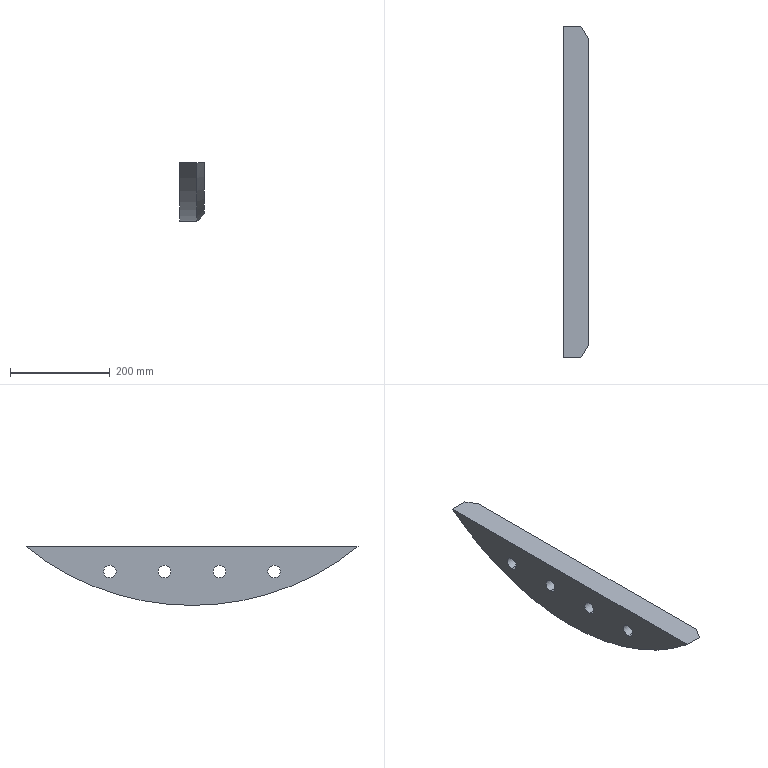Part | SolidWorks | features Chamfer 1, Extrusion 1, ICE 1 | 1 solid | 13 faces | box 50 x 666.801 x 118 mm | volume 2510197 mm3 | cylinder 9 | plane 3 | cone 1 | commonest cylinder face diameters 25 x8 1060 x1
STEP:
#1=CARTESIAN_POINT('',(-25.,-165.,-449.5));
#2=VERTEX_POINT('',#1);
#3=CARTESIAN_POINT('',(-25.,-165.,-474.5));
#4=VERTEX_POINT('',#3);
#5=CARTESIAN_POINT('',(-25.,-165.,-462.));
#6=DIRECTION('',(1.,0.,0.));
#7=DIRECTION('',(0.,0.,-1.));
#8=AXIS2_PLACEMENT_3D('',#5,#6,#7);
#9=CIRCLE('',#8,12.5);
#10=EDGE_CURVE('',#2,#4,#9,.T.);
#11=ORIENTED_EDGE('',*,*,#10,.F.);
#12=CARTESIAN_POINT('',(25.,-165.,-449.5));
#13=VERTEX_POINT('',#12);
#14=CARTESIAN_POINT('',(-56.,-165.,-449.5));
#15=DIRECTION('',(1.,0.,0.));
#16=VECTOR('',#15,1000.);
#17=LINE('',#14,#16);
#18=EDGE_CURVE('',#2,#13,#17,.T.);
#19=ORIENTED_EDGE('',*,*,#18,.T.);
#20=CARTESIAN_POINT('',(25.,-165.,-474.5));
#21=VERTEX_POINT('',#20);
#22=CARTESIAN_POINT('',(25.,-165.,-462.));
#23=DIRECTION('',(1.,0.,0.));
#24=DIRECTION('',(0.,0.,-1.));
#25=AXIS2_PLACEMENT_3D('',#22,#23,#24);
#26=CIRCLE('',#25,12.5);
#27=EDGE_CURVE('',#13,#21,#26,.T.);
#28=ORIENTED_EDGE('',*,*,#27,.T.);
#29=CARTESIAN_POINT('',(-56.,-165.,-474.5));
#30=DIRECTION('',(1.,0.,0.));
#31=VECTOR('',#30,1000.);
#32=LINE('',#29,#31);
#33=EDGE_CURVE('',#4,#21,#32,.T.);
#34=ORIENTED_EDGE('',*,*,#33,.F.);
#35=EDGE_LOOP('',(#11,#19,#28,#34));
#36=FACE_OUTER_BOUND('',#35,.T.);
#37=CARTESIAN_POINT('',(-56.,-165.,-462.));
#38=DIRECTION('',(1.,0.,0.));
#39=DIRECTION('',(0.,0.,-1.));
#40=AXIS2_PLACEMENT_3D('',#37,#38,#39);
#41=CYLINDRICAL_SURFACE('',#40,12.5);
#42=ADVANCED_FACE('',(#36),#41,.F.);
#43=CARTESIAN_POINT('',(-25.,165.,-449.5));
#44=VERTEX_POINT('',#43);
#45=CARTESIAN_POINT('',(-25.,165.,-474.5));
#46=VERTEX_POINT('',#45);
#47=CARTESIAN_POINT('',(-25.,165.,-462.));
#48=DIRECTION('',(1.,0.,0.));
#49=DIRECTION('',(0.,0.,-1.));
#50=AXIS2_PLACEMENT_3D('',#47,#48,#49);
#51=CIRCLE('',#50,12.5);
#52=EDGE_CURVE('',#44,#46,#51,.T.);
#53=ORIENTED_EDGE('',*,*,#52,.F.);
#54=CARTESIAN_POINT('',(25.,165.,-449.5));
#55=VERTEX_POINT('',#54);
#56=CARTESIAN_POINT('',(-56.,165.,-449.5));
#57=DIRECTION('',(1.,0.,0.));
#58=VECTOR('',#57,1000.);
#59=LINE('',#56,#58);
#60=EDGE_CURVE('',#44,#55,#59,.T.);
#61=ORIENTED_EDGE('',*,*,#60,.T.);
#62=CARTESIAN_POINT('',(25.,165.,-474.5));
#63=VERTEX_POINT('',#62);
#64=CARTESIAN_POINT('',(25.,165.,-462.));
#65=DIRECTION('',(1.,0.,0.));
#66=DIRECTION('',(0.,0.,-1.));
#67=AXIS2_PLACEMENT_3D('',#64,#65,#66);
#68=CIRCLE('',#67,12.5);
#69=EDGE_CURVE('',#55,#63,#68,.T.);
#70=ORIENTED_EDGE('',*,*,#69,.T.);
#71=CARTESIAN_POINT('',(-56.,165.,-474.5));
#72=DIRECTION('',(1.,0.,0.));
#73=VECTOR('',#72,1000.);
#74=LINE('',#71,#73);
#75=EDGE_CURVE('',#46,#63,#74,.T.);
#76=ORIENTED_EDGE('',*,*,#75,.F.);
#77=EDGE_LOOP('',(#53,#61,#70,#76));
#78=FACE_OUTER_BOUND('',#77,.T.);
#79=CARTESIAN_POINT('',(-56.,165.,-462.));
#80=DIRECTION('',(1.,0.,0.));
#81=DIRECTION('',(0.,0.,-1.));
#82=AXIS2_PLACEMENT_3D('',#79,#80,#81);
#83=CYLINDRICAL_SURFACE('',#82,12.5);
#84=ADVANCED_FACE('',(#78),#83,.F.);
#85=CARTESIAN_POINT('',(-25.,-55.,-449.5));
#86=VERTEX_POINT('',#85);
#87=CARTESIAN_POINT('',(-25.,-55.,-474.5));
#88=VERTEX_POINT('',#87);
#89=CARTESIAN_POINT('',(-25.,-55.,-462.));
#90=DIRECTION('',(1.,0.,0.));
#91=DIRECTION('',(0.,0.,-1.));
#92=AXIS2_PLACEMENT_3D('',#89,#90,#91);
#93=CIRCLE('',#92,12.5);
#94=EDGE_CURVE('',#86,#88,#93,.T.);
#95=ORIENTED_EDGE('',*,*,#94,.F.);
#96=CARTESIAN_POINT('',(25.,-55.,-449.5));
#97=VERTEX_POINT('',#96);
#98=CARTESIAN_POINT('',(-56.,-55.,-449.5));
#99=DIRECTION('',(1.,0.,0.));
#100=VECTOR('',#99,1000.);
#101=LINE('',#98,#100);
#102=EDGE_CURVE('',#86,#97,#101,.T.);
#103=ORIENTED_EDGE('',*,*,#102,.T.);
#104=CARTESIAN_POINT('',(25.,-55.,-474.5));
#105=VERTEX_POINT('',#104);
#106=CARTESIAN_POINT('',(25.,-55.,-462.));
#107=DIRECTION('',(1.,0.,0.));
#108=DIRECTION('',(0.,0.,-1.));
#109=AXIS2_PLACEMENT_3D('',#106,#107,#108);
#110=CIRCLE('',#109,12.5);
#111=EDGE_CURVE('',#97,#105,#110,.T.);
#112=ORIENTED_EDGE('',*,*,#111,.T.);
#113=CARTESIAN_POINT('',(-56.,-55.,-474.5));
#114=DIRECTION('',(1.,0.,0.));
#115=VECTOR('',#114,1000.);
#116=LINE('',#113,#115);
#117=EDGE_CURVE('',#88,#105,#116,.T.);
#118=ORIENTED_EDGE('',*,*,#117,.F.);
#119=EDGE_LOOP('',(#95,#103,#112,#118));
#120=FACE_OUTER_BOUND('',#119,.T.);
#121=CARTESIAN_POINT('',(-56.,-55.,-462.));
#122=DIRECTION('',(1.,0.,0.));
#123=DIRECTION('',(0.,0.,-1.));
#124=AXIS2_PLACEMENT_3D('',#121,#122,#123);
#125=CYLINDRICAL_SURFACE('',#124,12.5);
#126=ADVANCED_FACE('',(#120),#125,.F.);
#127=CARTESIAN_POINT('',(-25.,55.,-449.5));
#128=VERTEX_POINT('',#127);
#129=CARTESIAN_POINT('',(-25.,55.,-474.5));
#130=VERTEX_POINT('',#129);
#131=CARTESIAN_POINT('',(-25.,55.,-462.));
#132=DIRECTION('',(1.,0.,0.));
#133=DIRECTION('',(0.,0.,-1.));
#134=AXIS2_PLACEMENT_3D('',#131,#132,#133);
#135=CIRCLE('',#134,12.5);
#136=EDGE_CURVE('',#128,#130,#135,.T.);
#137=ORIENTED_EDGE('',*,*,#136,.F.);
#138=CARTESIAN_POINT('',(25.,55.,-449.5));
#139=VERTEX_POINT('',#138);
#140=CARTESIAN_POINT('',(-56.,55.,-449.5));
#141=DIRECTION('',(1.,0.,0.));
#142=VECTOR('',#141,1000.);
#143=LINE('',#140,#142);
#144=EDGE_CURVE('',#128,#139,#143,.T.);
#145=ORIENTED_EDGE('',*,*,#144,.T.);
#146=CARTESIAN_POINT('',(25.,55.,-474.5));
#147=VERTEX_POINT('',#146);
#148=CARTESIAN_POINT('',(25.,55.,-462.));
#149=DIRECTION('',(1.,0.,0.));
#150=DIRECTION('',(0.,0.,-1.));
#151=AXIS2_PLACEMENT_3D('',#148,#149,#150);
#152=CIRCLE('',#151,12.5);
#153=EDGE_CURVE('',#139,#147,#152,.T.);
#154=ORIENTED_EDGE('',*,*,#153,.T.);
#155=CARTESIAN_POINT('',(-56.,55.,-474.5));
#156=DIRECTION('',(1.,0.,0.));
#157=VECTOR('',#156,1000.);
#158=LINE('',#155,#157);
#159=EDGE_CURVE('',#130,#147,#158,.T.);
#160=ORIENTED_EDGE('',*,*,#159,.F.);
#161=EDGE_LOOP('',(#137,#145,#154,#160));
#162=FACE_OUTER_BOUND('',#161,.T.);
#163=CARTESIAN_POINT('',(-56.,55.,-462.));
#164=DIRECTION('',(1.,0.,0.));
#165=DIRECTION('',(0.,0.,-1.));
#166=AXIS2_PLACEMENT_3D('',#163,#164,#165);
#167=CYLINDRICAL_SURFACE('',#166,12.5);
#168=ADVANCED_FACE('',(#162),#167,.F.);
#169=CARTESIAN_POINT('',(10.,333.401,-412.));
#170=VERTEX_POINT('',#169);
#171=CARTESIAN_POINT('',(-25.,333.401,-412.));
#172=VERTEX_POINT('',#171);
#173=CARTESIAN_POINT('',(25.,333.401,-412.));
#174=DIRECTION('',(-1.,0.,0.));
#175=VECTOR('',#174,1000.);
#176=LINE('',#173,#175);
#177=EDGE_CURVE('',#170,#172,#176,.T.);
#178=ORIENTED_EDGE('',*,*,#177,.F.);
#179=CARTESIAN_POINT('',(10.,-333.401,-412.));
#180=VERTEX_POINT('',#179);
#181=CARTESIAN_POINT('',(10.,0.,0.));
#182=DIRECTION('',(-1.,0.,0.));
#183=DIRECTION('',(0.,0.,-1.));
#184=AXIS2_PLACEMENT_3D('',#181,#182,#183);
#185=CIRCLE('',#184,530.);
#186=EDGE_CURVE('',#170,#180,#185,.T.);
#187=ORIENTED_EDGE('',*,*,#186,.T.);
#188=CARTESIAN_POINT('',(-25.,-333.401,-412.));
#189=VERTEX_POINT('',#188);
#190=CARTESIAN_POINT('',(25.,-333.401,-412.));
#191=DIRECTION('',(-1.,0.,0.));
#192=VECTOR('',#191,1000.);
#193=LINE('',#190,#192);
#194=EDGE_CURVE('',#180,#189,#193,.T.);
#195=ORIENTED_EDGE('',*,*,#194,.T.);
#196=CARTESIAN_POINT('',(-25.,0.,0.));
#197=DIRECTION('',(1.,0.,0.));
#198=DIRECTION('',(0.,0.,-1.));
#199=AXIS2_PLACEMENT_3D('',#196,#197,#198);
#200=CIRCLE('',#199,530.);
#201=EDGE_CURVE('',#189,#172,#200,.T.);
#202=ORIENTED_EDGE('',*,*,#201,.T.);
#203=EDGE_LOOP('',(#178,#187,#195,#202));
#204=FACE_OUTER_BOUND('',#203,.T.);
#205=CARTESIAN_POINT('',(25.,0.,0.));
#206=DIRECTION('',(-1.,0.,0.));
#207=DIRECTION('',(0.,0.,1.));
#208=AXIS2_PLACEMENT_3D('',#205,#206,#207);
#209=CYLINDRICAL_SURFACE('',#208,530.);
#210=ADVANCED_FACE('',(#204),#209,.T.);
#211=CARTESIAN_POINT('',(25.,309.,-412.));
#212=VERTEX_POINT('',#211);
#213=CARTESIAN_POINT('',(25.,-309.,-412.));
#214=VERTEX_POINT('',#213);
#215=CARTESIAN_POINT('',(25.,333.401,-412.));
#216=DIRECTION('',(0.,-1.,0.));
#217=VECTOR('',#216,1000.);
#218=LINE('',#215,#217);
#219=EDGE_CURVE('',#212,#214,#218,.T.);
#220=ORIENTED_EDGE('',*,*,#219,.F.);
#221=CARTESIAN_POINT('',(25.,309.,-412.));
#222=CARTESIAN_POINT('',(20.088,317.187,-412.));
#223=CARTESIAN_POINT('',(15.084,325.319,-412.));
#224=CARTESIAN_POINT('',(10.,333.401,-412.));
#225=B_SPLINE_CURVE_WITH_KNOTS('',3,(#221,#222,#223,#224),.UNSPECIFIED.,.F.,.F.,(4,4),(0.,0.02864),.UNSPECIFIED.);
#226=EDGE_CURVE('',#212,#170,#225,.T.);
#227=ORIENTED_EDGE('',*,*,#226,.T.);
#228=ORIENTED_EDGE('',*,*,#177,.T.);
#229=CARTESIAN_POINT('',(-25.,333.401,-412.));
#230=DIRECTION('',(0.,-1.,0.));
#231=VECTOR('',#230,1000.);
#232=LINE('',#229,#231);
#233=EDGE_CURVE('',#172,#189,#232,.T.);
#234=ORIENTED_EDGE('',*,*,#233,.T.);
#235=ORIENTED_EDGE('',*,*,#194,.F.);
#236=CARTESIAN_POINT('',(10.,-333.401,-412.));
#237=CARTESIAN_POINT('',(15.084,-325.319,-412.));
#238=CARTESIAN_POINT('',(20.088,-317.187,-412.));
#239=CARTESIAN_POINT('',(25.,-309.,-412.));
#240=B_SPLINE_CURVE_WITH_KNOTS('',3,(#236,#237,#238,#239),.UNSPECIFIED.,.F.,.F.,(4,4),(0.,0.02864),.UNSPECIFIED.);
#241=EDGE_CURVE('',#180,#214,#240,.T.);
#242=ORIENTED_EDGE('',*,*,#241,.T.);
#243=EDGE_LOOP('',(#220,#227,#228,#234,#235,#242));
#244=FACE_OUTER_BOUND('',#243,.T.);
#245=CARTESIAN_POINT('',(25.,333.401,-412.));
#246=DIRECTION('',(0.,0.,-1.));
#247=DIRECTION('',(-1.,0.,0.));
#248=AXIS2_PLACEMENT_3D('',#245,#246,#247);
#249=PLANE('',#248);
#250=ADVANCED_FACE('',(#244),#249,.F.);
#251=CARTESIAN_POINT('',(25.,-165.,-462.));
#252=DIRECTION('',(1.,0.,0.));
#253=DIRECTION('',(0.,0.,-1.));
#254=AXIS2_PLACEMENT_3D('',#251,#252,#253);
#255=CIRCLE('',#254,12.5);
#256=EDGE_CURVE('',#21,#13,#255,.T.);
#257=ORIENTED_EDGE('',*,*,#256,.F.);
#258=ORIENTED_EDGE('',*,*,#27,.F.);
#259=EDGE_LOOP('',(#257,#258));
#260=FACE_BOUND('',#259,.T.);
#261=CARTESIAN_POINT('',(25.,165.,-462.));
#262=DIRECTION('',(1.,0.,0.));
#263=DIRECTION('',(0.,0.,-1.));
#264=AXIS2_PLACEMENT_3D('',#261,#262,#263);
#265=CIRCLE('',#264,12.5);
#266=EDGE_CURVE('',#63,#55,#265,.T.);
#267=ORIENTED_EDGE('',*,*,#266,.F.);
#268=ORIENTED_EDGE('',*,*,#69,.F.);
#269=EDGE_LOOP('',(#267,#268));
#270=FACE_BOUND('',#269,.T.);
#271=CARTESIAN_POINT('',(25.,-55.,-462.));
#272=DIRECTION('',(1.,0.,0.));
#273=DIRECTION('',(0.,0.,-1.));
#274=AXIS2_PLACEMENT_3D('',#271,#272,#273);
#275=CIRCLE('',#274,12.5);
#276=EDGE_CURVE('',#105,#97,#275,.T.);
#277=ORIENTED_EDGE('',*,*,#276,.F.);
#278=ORIENTED_EDGE('',*,*,#111,.F.);
#279=EDGE_LOOP('',(#277,#278));
#280=FACE_BOUND('',#279,.T.);
#281=CARTESIAN_POINT('',(25.,55.,-462.));
#282=DIRECTION('',(1.,0.,0.));
#283=DIRECTION('',(0.,0.,-1.));
#284=AXIS2_PLACEMENT_3D('',#281,#282,#283);
#285=CIRCLE('',#284,12.5);
#286=EDGE_CURVE('',#147,#139,#285,.T.);
#287=ORIENTED_EDGE('',*,*,#286,.F.);
#288=ORIENTED_EDGE('',*,*,#153,.F.);
#289=EDGE_LOOP('',(#287,#288));
#290=FACE_BOUND('',#289,.T.);
#291=ORIENTED_EDGE('',*,*,#219,.T.);
#292=CARTESIAN_POINT('',(25.,0.,0.));
#293=DIRECTION('',(1.,0.,0.));
#294=DIRECTION('',(0.,0.,-1.));
#295=AXIS2_PLACEMENT_3D('',#292,#293,#294);
#296=CIRCLE('',#295,515.);
#297=EDGE_CURVE('',#214,#212,#296,.T.);
#298=ORIENTED_EDGE('',*,*,#297,.T.);
#299=EDGE_LOOP('',(#291,#298));
#300=FACE_OUTER_BOUND('',#299,.T.);
#301=CARTESIAN_POINT('',(25.,0.,0.));
#302=DIRECTION('',(1.,0.,0.));
#303=DIRECTION('',(0.,0.,-1.));
#304=AXIS2_PLACEMENT_3D('',#301,#302,#303);
#305=PLANE('',#304);
#306=ADVANCED_FACE('',(#260,#270,#280,#290,#300),#305,.T.);
#307=CARTESIAN_POINT('',(-25.,-165.,-462.));
#308=DIRECTION('',(1.,0.,0.));
#309=DIRECTION('',(0.,0.,-1.));
#310=AXIS2_PLACEMENT_3D('',#307,#308,#309);
#311=CIRCLE('',#310,12.5);
#312=EDGE_CURVE('',#4,#2,#311,.T.);
#313=ORIENTED_EDGE('',*,*,#312,.T.);
#314=ORIENTED_EDGE('',*,*,#10,.T.);
#315=EDGE_LOOP('',(#313,#314));
#316=FACE_BOUND('',#315,.T.);
#317=CARTESIAN_POINT('',(-25.,165.,-462.));
#318=DIRECTION('',(1.,0.,0.));
#319=DIRECTION('',(0.,0.,-1.));
#320=AXIS2_PLACEMENT_3D('',#317,#318,#319);
#321=CIRCLE('',#320,12.5);
#322=EDGE_CURVE('',#46,#44,#321,.T.);
#323=ORIENTED_EDGE('',*,*,#322,.T.);
#324=ORIENTED_EDGE('',*,*,#52,.T.);
#325=EDGE_LOOP('',(#323,#324));
#326=FACE_BOUND('',#325,.T.);
#327=CARTESIAN_POINT('',(-25.,-55.,-462.));
#328=DIRECTION('',(1.,0.,0.));
#329=DIRECTION('',(0.,0.,-1.));
#330=AXIS2_PLACEMENT_3D('',#327,#328,#329);
#331=CIRCLE('',#330,12.5);
#332=EDGE_CURVE('',#88,#86,#331,.T.);
#333=ORIENTED_EDGE('',*,*,#332,.T.);
#334=ORIENTED_EDGE('',*,*,#94,.T.);
#335=EDGE_LOOP('',(#333,#334));
#336=FACE_BOUND('',#335,.T.);
#337=CARTESIAN_POINT('',(-25.,55.,-462.));
#338=DIRECTION('',(1.,0.,0.));
#339=DIRECTION('',(0.,0.,-1.));
#340=AXIS2_PLACEMENT_3D('',#337,#338,#339);
#341=CIRCLE('',#340,12.5);
#342=EDGE_CURVE('',#130,#128,#341,.T.);
#343=ORIENTED_EDGE('',*,*,#342,.T.);
#344=ORIENTED_EDGE('',*,*,#136,.T.);
#345=EDGE_LOOP('',(#343,#344));
#346=FACE_BOUND('',#345,.T.);
#347=ORIENTED_EDGE('',*,*,#201,.F.);
#348=ORIENTED_EDGE('',*,*,#233,.F.);
#349=EDGE_LOOP('',(#347,#348));
#350=FACE_OUTER_BOUND('',#349,.T.);
#351=CARTESIAN_POINT('',(-25.,0.,0.));
#352=DIRECTION('',(1.,0.,0.));
#353=DIRECTION('',(0.,0.,-1.));
#354=AXIS2_PLACEMENT_3D('',#351,#352,#353);
#355=PLANE('',#354);
#356=ADVANCED_FACE('',(#316,#326,#336,#346,#350),#355,.F.);
#357=ORIENTED_EDGE('',*,*,#144,.F.);
#358=ORIENTED_EDGE('',*,*,#342,.F.);
#359=ORIENTED_EDGE('',*,*,#159,.T.);
#360=ORIENTED_EDGE('',*,*,#286,.T.);
#361=EDGE_LOOP('',(#357,#358,#359,#360));
#362=FACE_OUTER_BOUND('',#361,.T.);
#363=CARTESIAN_POINT('',(-56.,55.,-462.));
#364=DIRECTION('',(1.,0.,0.));
#365=DIRECTION('',(0.,0.,-1.));
#366=AXIS2_PLACEMENT_3D('',#363,#364,#365);
#367=CYLINDRICAL_SURFACE('',#366,12.5);
#368=ADVANCED_FACE('',(#362),#367,.F.);
#369=ORIENTED_EDGE('',*,*,#102,.F.);
#370=ORIENTED_EDGE('',*,*,#332,.F.);
#371=ORIENTED_EDGE('',*,*,#117,.T.);
#372=ORIENTED_EDGE('',*,*,#276,.T.);
#373=EDGE_LOOP('',(#369,#370,#371,#372));
#374=FACE_OUTER_BOUND('',#373,.T.);
#375=CARTESIAN_POINT('',(-56.,-55.,-462.));
#376=DIRECTION('',(1.,0.,0.));
#377=DIRECTION('',(0.,0.,-1.));
#378=AXIS2_PLACEMENT_3D('',#375,#376,#377);
#379=CYLINDRICAL_SURFACE('',#378,12.5);
#380=ADVANCED_FACE('',(#374),#379,.F.);
#381=ORIENTED_EDGE('',*,*,#60,.F.);
#382=ORIENTED_EDGE('',*,*,#322,.F.);
#383=ORIENTED_EDGE('',*,*,#75,.T.);
#384=ORIENTED_EDGE('',*,*,#266,.T.);
#385=EDGE_LOOP('',(#381,#382,#383,#384));
#386=FACE_OUTER_BOUND('',#385,.T.);
#387=CARTESIAN_POINT('',(-56.,165.,-462.));
#388=DIRECTION('',(1.,0.,0.));
#389=DIRECTION('',(0.,0.,-1.));
#390=AXIS2_PLACEMENT_3D('',#387,#388,#389);
#391=CYLINDRICAL_SURFACE('',#390,12.5);
#392=ADVANCED_FACE('',(#386),#391,.F.);
#393=ORIENTED_EDGE('',*,*,#18,.F.);
#394=ORIENTED_EDGE('',*,*,#312,.F.);
#395=ORIENTED_EDGE('',*,*,#33,.T.);
#396=ORIENTED_EDGE('',*,*,#256,.T.);
#397=EDGE_LOOP('',(#393,#394,#395,#396));
#398=FACE_OUTER_BOUND('',#397,.T.);
#399=CARTESIAN_POINT('',(-56.,-165.,-462.));
#400=DIRECTION('',(1.,0.,0.));
#401=DIRECTION('',(0.,0.,-1.));
#402=AXIS2_PLACEMENT_3D('',#399,#400,#401);
#403=CYLINDRICAL_SURFACE('',#402,12.5);
#404=ADVANCED_FACE('',(#398),#403,.F.);
#405=ORIENTED_EDGE('',*,*,#241,.F.);
#406=ORIENTED_EDGE('',*,*,#186,.F.);
#407=ORIENTED_EDGE('',*,*,#226,.F.);
#408=ORIENTED_EDGE('',*,*,#297,.F.);
#409=EDGE_LOOP('',(#405,#406,#407,#408));
#410=FACE_OUTER_BOUND('',#409,.T.);
#411=CARTESIAN_POINT('',(25.,0.,0.));
#412=DIRECTION('',(-1.,0.,0.));
#413=DIRECTION('',(0.,0.,1.));
#414=AXIS2_PLACEMENT_3D('',#411,#412,#413);
#415=CONICAL_SURFACE('',#414,515.,0.7854);
#416=ADVANCED_FACE('',(#410),#415,.T.);
#417=CLOSED_SHELL('',(#42,#84,#126,#168,#210,#250,#306,#356,#368,#380,#392,#404,#416));
#418=MANIFOLD_SOLID_BREP('',#417);
#419=CARTESIAN_POINT('',(0.,0.,0.));
#420=DIRECTION('',(0.,0.,1.));
#421=DIRECTION('',(1.,0.,0.));
#422=AXIS2_PLACEMENT_3D('',#419,#420,#421);
#423=(LENGTH_UNIT()NAMED_UNIT(*)SI_UNIT(.MILLI.,.METRE.));
#424=UNCERTAINTY_MEASURE_WITH_UNIT(LENGTH_MEASURE(0.00001),#423,'','');
#425=(NAMED_UNIT(*)PLANE_ANGLE_UNIT()SI_UNIT($,.RADIAN.));
#426=(NAMED_UNIT(*)SI_UNIT($,.STERADIAN.)SOLID_ANGLE_UNIT());
#427=(GEOMETRIC_REPRESENTATION_CONTEXT(3)GLOBAL_UNCERTAINTY_ASSIGNED_CONTEXT((#424))GLOBAL_UNIT_ASSIGNED_CONTEXT((#423,#425,#426))REPRESENTATION_CONTEXT('',''));
#428=ADVANCED_BREP_SHAPE_REPRESENTATION('',(#418,#422),#427);